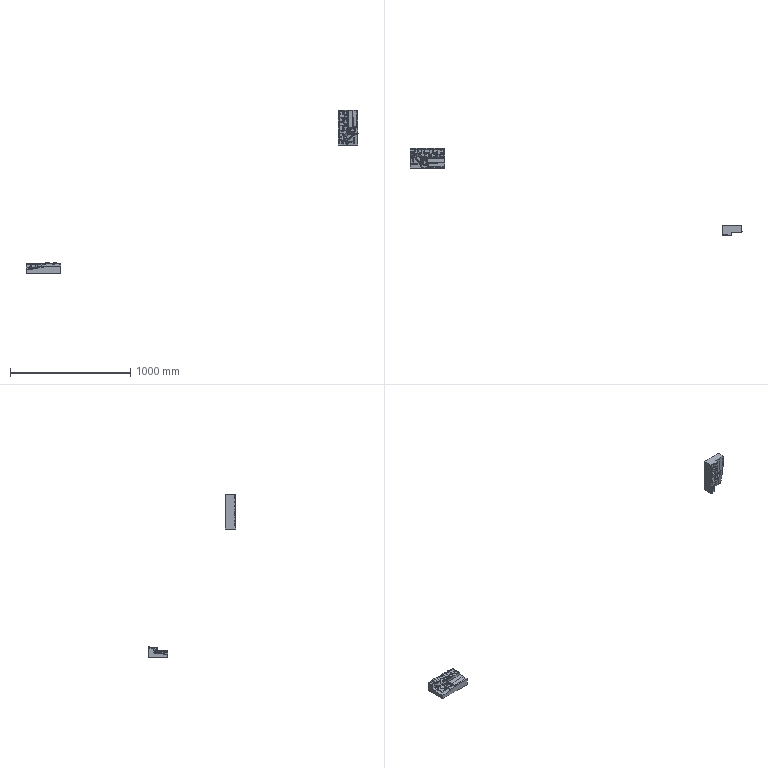NC program | NX | posted with a generic post | part box 2756 x 729.572 x 1353 mm
Lines 28320 to 29345 of 180527:
(CONTOUR_AREA , TOOL : B10)
N56626 M6
N56628 G54
N56630 G17 G0 G90 X35.48 Y166.497 B0. C0. S3000 M3
N56632 G43 Z10. H0
N56634 Z0.
N56636 G94 G1 Z-4.102 F2500.
N56638 X36.929 Z-4.118
N56640 X37.143 Z-3.988
N56642 X38.643 Z-3.197
N56644 X40.143 Z-2.553
N56646 X41.643 Z-2.051
N56648 X43.143 Z-1.669
N56650 X44.643 Z-1.416
N56652 X46.143 Z-1.275
N56654 X49.143 Z-1.261
N56656 X52.143 Z-1.295
N56658 X55.143 Z-1.329
N56660 X58.143 Z-1.363
N56662 X61.143 Z-1.397
N56664 X62.643 Z-1.472
N56666 X64.143 Z-1.658
N56668 X65.643 Z-1.962
N56670 X67.143 Z-2.389
N56672 X68.643 Z-2.946
N56674 X70.143 Z-3.648
N56676 X71.651 Z-4.513
N56678 X73.143 Z-4.527
N56680 X76.143 Z-4.554
N56682 X79.143 Z-4.582
N56684 X82.143 Z-4.609
N56686 X85.143 Z-4.636
N56688 X88.143 Z-4.658
N56690 X89.791 Z-4.669
N56692 X91.143 Z-3.943
N56694 X91.893 Z-3.62
N56696 X92.643 Z-3.368
N56698 X94.143 Z-3.051
N56700 X95.643 Z-2.951
N56702 X97.143 Z-2.899
N56704 X100.143 Z-2.794
N56706 X103.143 Z-2.689
N56708 X106.143 Z-2.584
N56710 X109.143 Z-2.479
N56712 X112.143 Z-2.374
N56714 X113.643 Z-2.321
N56716 X115.143 Z-2.344
N56718 X116.643 Z-2.59
N56720 X118.143 Z-3.015
N56722 X119.643 Z-3.57
N56724 X121.143 Z-4.268
N56726 X122.074 Z-4.782
N56728 X124.143 Z-4.78
N56730 X127.143 Z-4.777
N56732 X130.143 Z-4.775
N56734 X133.143 Z-4.772
N56736 X136.143 Z-4.764
N56738 X139.143 Z-4.755
N56740 X142.143 Z-4.746
N56742 X145.143 Z-4.733
N56744 X148.143 Z-4.717
N56746 X151.143 Z-4.702
N56748 X153.393 Z-4.691
N56750 X154.143 Z-4.668
N56752 X154.518 Z-4.517
N56754 X155.643 Z-3.508
N56756 X156.393 Z-2.935
N56758 X157.143 Z-2.443
N56760 X158.643 Z-1.654
N56762 X160.143 Z-1.097
N56764 X161.643 Z-0.737
N56766 X163.143 Z-0.56
N56768 X166.143 Z-0.475
N56770 X169.143 Z-0.401
N56772 X172.143 Z-0.333
N56774 X175.143 Z-0.266
N56776 X178.143 Z-0.204
N56778 X181.143 Z-0.144
N56780 X184.143 Z-0.085
N56782 X187.143 Z-0.027
N56784 X188.643 Z-0.001
N56786 X190.143 Z-0.078
N56788 X191.643 Z-0.328
N56790 X193.143 Z-0.762
N56792 X194.643 Z-1.408
N56794 X196.143 Z-2.302
N56796 X196.893 Z-2.858
N56798 X197.643 Z-3.51
N56800 X198.018 Z-3.87
N56802 X198.393 Z-4.171
N56804 X198.768 Z-4.281
N56806 X199.143 Z-4.283
N56808 X202.143 Z-4.269
N56810 X205.143 Z-4.26
N56812 X208.143 Z-4.251
N56814 X211.143 Z-4.242
N56816 X214.143 Z-4.232
N56818 X217.143 Z-4.223
N56820 X219.393 Z-4.215
N56822 X219.768 Z-4.122
N56824 X220.143 Z-3.84
N56826 X220.893 Z-3.116
N56828 X221.643 Z-2.476
N56830 X222.393 Z-1.935
N56832 X223.143 Z-1.484
N56834 X223.893 Z-1.112
N56836 X224.643 Z-0.809
N56838 X226.143 Z-0.378
N56840 X227.643 Z-0.165
N56842 X229.143 Z-0.144
N56844 X232.143 Z-0.177
N56846 X235.143 Z-0.211
N56848 X238.143 Z-0.25
N56850 X241.143 Z-0.289
N56852 X244.143 Z-0.332
N56854 X247.143 Z-0.379
N56856 X250.143 Z-0.426
N56858 X253.143 Z-0.474
N56860 X254.643 Z-0.515
N56862 X256.143 Z-0.727
N56864 X257.643 Z-1.164
N56866 X258.393 Z-1.469
N56868 X259.143 Z-1.842
N56870 X259.893 Z-2.294
N56872 X260.643 Z-2.836
N56874 X261.393 Z-3.481
N56876 X262.143 Z-4.212
N56878 X262.518 Z-4.441
N56880 X262.893 Z-4.497
N56882 X265.143 Z-4.53
N56884 X268.143 Z-4.577
N56886 X271.143 Z-4.624
N56888 X274.143 Z-4.672
N56890 X277.143 Z-4.719
N56892 X280.143 Z-4.767
N56894 X283.143
N56896 X286.143
N56898 X288.497 Z-4.768
N56900 X288.498 Y166.301
N56902 X286.143 Z-4.767
N56904 X283.143
N56906 X280.143
N56908 X277.143 Z-4.719
N56910 X274.143 Z-4.672
N56912 X271.143 Z-4.625
N56914 X268.143 Z-4.577
N56916 X265.143 Z-4.53
N56918 X263.643 Z-4.509
N56920 X262.893 Z-4.497
N56922 X262.518 Z-4.441
N56924 X262.143 Z-4.212
N56926 X261.393 Z-3.481
N56928 X260.643 Z-2.836
N56930 X259.893 Z-2.294
N56932 X259.143 Z-1.842
N56934 X258.393 Z-1.469
N56936 X257.643 Z-1.164
N56938 X256.143 Z-0.727
N56940 X254.643 Z-0.515
N56942 X253.143 Z-0.474
N56944 X250.143 Z-0.426
N56946 X247.143 Z-0.379
N56948 X244.143 Z-0.332
N56950 X241.143 Z-0.289
N56952 X238.143 Z-0.25
N56954 X235.143 Z-0.211
N56956 X232.143 Z-0.177
N56958 X229.143 Z-0.144
N56960 X227.643 Z-0.165
N56962 X226.143 Z-0.378
N56964 X224.643 Z-0.809
N56966 X223.893 Z-1.112
N56968 X223.143 Z-1.484
N56970 X222.393 Z-1.935
N56972 X221.643 Z-2.476
N56974 X220.893 Z-3.117
N56976 X220.143 Z-3.84
N56978 X219.768 Z-4.122
N56980 X219.393 Z-4.214
N56982 X218.643 Z-4.221
N56984 X217.143 Z-4.223
N56986 X214.143 Z-4.232
N56988 X211.143 Z-4.242
N56990 X208.143 Z-4.251
N56992 X205.143 Z-4.26
N56994 X202.143 Z-4.269
N56996 X199.143 Z-4.283
N56998 X198.768 Z-4.281
N57000 X198.393 Z-4.171
N57002 X198.018 Z-3.87
N57004 X197.643 Z-3.51
N57006 X196.893 Z-2.858
N57008 X196.143 Z-2.302
N57010 X194.643 Z-1.408
N57012 X193.143 Z-0.762
N57014 X191.643 Z-0.328
N57016 X190.143 Z-0.078
N57018 X188.643 Z-0.001
N57020 X187.143 Z-0.027
N57022 X184.143 Z-0.085
N57024 X181.143 Z-0.144
N57026 X178.143 Z-0.204
N57028 X175.143 Z-0.266
N57030 X172.143 Z-0.333
N57032 X169.143 Z-0.401
N57034 X166.143 Z-0.474
N57036 X163.143 Z-0.56
N57038 X161.643 Z-0.737
N57040 X160.143 Z-1.097
N57042 X158.643 Z-1.654
N57044 X157.143 Z-2.443
N57046 X156.393 Z-2.935
N57048 X155.643 Z-3.508
N57050 X154.893 Z-4.184
N57052 X154.518 Z-4.517
N57054 X154.143 Z-4.668
N57056 X153.393 Z-4.691
N57058 X152.643 Z-4.695
N57060 X151.143 Z-4.702
N57062 X148.143 Z-4.717
N57064 X145.143 Z-4.733
N57066 X142.143 Z-4.746
N57068 X139.143 Z-4.755
N57070 X136.143 Z-4.764
N57072 X133.143 Z-4.772
N57074 X130.143 Z-4.775
N57076 X127.143 Z-4.777
N57078 X124.143 Z-4.78
N57080 X122.074 Z-4.782
N57082 X121.143 Z-4.268
N57084 X119.643 Z-3.57
N57086 X118.143 Z-3.015
N57088 X116.643 Z-2.59
N57090 X115.143 Z-2.344
N57092 X113.643 Z-2.321
N57094 X112.143 Z-2.374
N57096 X109.143 Z-2.479
N57098 X106.143 Z-2.584
N57100 X103.143 Z-2.689
N57102 X100.143 Z-2.794
N57104 X97.143 Z-2.899
N57106 X95.643 Z-2.951
N57108 X94.143 Z-3.051
N57110 X92.643 Z-3.368
N57112 X91.893 Z-3.62
N57114 X91.143 Z-3.943
N57116 X89.791 Z-4.669
N57118 X88.143 Z-4.658
N57120 X85.143 Z-4.636
N57122 X82.143 Z-4.609
N57124 X79.143 Z-4.582
N57126 X76.143 Z-4.554
N57128 X73.143 Z-4.527
N57130 X71.651 Z-4.513
N57132 X70.143 Z-3.648
N57134 X68.643 Z-2.946
N57136 X67.143 Z-2.389
N57138 X65.643 Z-1.962
N57140 X64.143 Z-1.658
N57142 X62.643 Z-1.472
N57144 X61.143 Z-1.397
N57146 X58.143 Z-1.363
N57148 X55.143 Z-1.329
N57150 X52.143 Z-1.295
N57152 X49.143 Z-1.261
N57154 X46.143 Z-1.275
N57156 X44.643 Z-1.416
N57158 X43.143 Z-1.669
N57160 X41.643 Z-2.051
N57162 X40.143 Z-2.553
N57164 X38.643 Z-3.197
N57166 X37.143 Z-3.988
N57168 X36.929 Z-4.118
N57170 X34.143 Z-4.086
N57172 X31.143 Z-4.052
N57174 X28.143 Z-4.017
N57176 X25.143 Z-3.983
N57178 X22.143 Z-3.948
N57180 X19.143 Z-3.913
N57182 X16.143 Z-3.879
N57184 X13.143 Z-3.844
N57186 X10.143 Z-3.809
N57188 X7.143 Z-3.775
N57190 X4.143 Z-3.74
N57192 X1.143 Z-3.705
N57194 X-1.797 Z-3.671
N57196 X-1.857
N57198 Y166.103
N57200 X-1.797
N57202 X1.143 Z-3.705
N57204 X4.143 Z-3.74
N57206 X7.143 Z-3.775
N57208 X10.143 Z-3.809
N57210 X13.143 Z-3.844
N57212 X16.143 Z-3.879
N57214 X19.143 Z-3.913
N57216 X22.143 Z-3.948
N57218 X25.143 Z-3.983
N57220 X28.143 Z-4.017
N57222 X31.143 Z-4.052
N57224 X34.143 Z-4.086
N57226 X36.929 Z-4.118
N57228 X37.143 Z-3.988
N57230 X38.643 Z-3.197
N57232 X40.143 Z-2.553
N57234 X41.643 Z-2.051
N57236 X43.143 Z-1.669
N57238 X44.643 Z-1.416
N57240 X46.143 Z-1.275
N57242 X49.143 Z-1.261
N57244 X52.143 Z-1.295
N57246 X55.143 Z-1.329
N57248 X58.143 Z-1.363
N57250 X61.143 Z-1.397
N57252 X62.643 Z-1.472
N57254 X64.143 Z-1.658
N57256 X65.643 Z-1.962
N57258 X67.143 Z-2.389
N57260 X68.643 Z-2.946
N57262 X70.143 Z-3.648
N57264 X71.651 Z-4.513
N57266 X73.143 Z-4.527
N57268 X76.143 Z-4.554
N57270 X79.143 Z-4.582
N57272 X82.143 Z-4.609
N57274 X85.143 Z-4.636
N57276 X88.143 Z-4.658
N57278 X89.791 Z-4.669
N57280 X91.143 Z-3.943
N57282 X91.893 Z-3.62
N57284 X92.643 Z-3.368
N57286 X94.143 Z-3.051
N57288 X95.643 Z-2.951
N57290 X97.143 Z-2.899
N57292 X100.143 Z-2.794
N57294 X103.143 Z-2.689
N57296 X106.143 Z-2.584
N57298 X109.143 Z-2.479
N57300 X112.143 Z-2.374
N57302 X113.643 Z-2.321
N57304 X115.143 Z-2.344
N57306 X116.643 Z-2.59
N57308 X118.143 Z-3.015
N57310 X119.643 Z-3.57
N57312 X121.143 Z-4.268
N57314 X122.074 Z-4.782
N57316 X124.143 Z-4.78
N57318 X127.143 Z-4.777
N57320 X130.143 Z-4.775
N57322 X133.143 Z-4.772
N57324 X136.143 Z-4.764
N57326 X139.143 Z-4.755
N57328 X142.143 Z-4.746
N57330 X145.143 Z-4.733
N57332 X148.143 Z-4.717
N57334 X151.143 Z-4.702
N57336 X153.393 Z-4.691
N57338 X154.143 Z-4.668
N57340 X154.518 Z-4.517
N57342 X154.893 Z-4.184
N57344 X155.643 Z-3.508
N57346 X156.393 Z-2.935
N57348 X157.143 Z-2.443
N57350 X158.643 Z-1.654
N57352 X160.143 Z-1.097
N57354 X161.643 Z-0.737
N57356 X163.143 Z-0.56
N57358 X166.143 Z-0.474
N57360 X169.143 Z-0.401
N57362 X172.143 Z-0.333
N57364 X175.143 Z-0.266
N57366 X178.143 Z-0.204
N57368 X181.143 Z-0.144
N57370 X184.143 Z-0.085
N57372 X187.143 Z-0.027
N57374 X188.643 Z-0.001
N57376 X190.143 Z-0.078
N57378 X191.643 Z-0.328
N57380 X193.143 Z-0.762
N57382 X194.643 Z-1.408
N57384 X196.143 Z-2.302
N57386 X196.893 Z-2.858
N57388 X197.643 Z-3.51
N57390 X198.018 Z-3.87
N57392 X198.393 Z-4.171
N57394 X198.768 Z-4.281
N57396 X199.143 Z-4.283
N57398 X202.143 Z-4.269
N57400 X205.143 Z-4.26
N57402 X208.143 Z-4.251
N57404 X211.143 Z-4.242
N57406 X214.143 Z-4.232
N57408 X217.143 Z-4.223
N57410 X218.643 Z-4.221
N57412 X219.393 Z-4.214
N57414 X219.768 Z-4.122
N57416 X220.143 Z-3.84
N57418 X220.893 Z-3.117
N57420 X221.643 Z-2.476
N57422 X222.393 Z-1.935
N57424 X223.143 Z-1.484
N57426 X223.893 Z-1.112
N57428 X224.643 Z-0.809
N57430 X226.143 Z-0.378
N57432 X227.643 Z-0.165
N57434 X229.143 Z-0.144
N57436 X232.143 Z-0.177
N57438 X235.143 Z-0.211
N57440 X238.143 Z-0.25
N57442 X241.143 Z-0.288
N57444 X244.143 Z-0.332
N57446 X247.143 Z-0.379
N57448 X250.143 Z-0.426
N57450 X253.143 Z-0.474
N57452 X254.643 Z-0.515
N57454 X256.143 Z-0.727
N57456 X257.643 Z-1.164
N57458 X258.393 Z-1.469
N57460 X259.143 Z-1.842
N57462 X259.893 Z-2.294
N57464 X260.643 Z-2.836
N57466 X261.393 Z-3.481
N57468 X262.143 Z-4.212
N57470 X262.518 Z-4.441
N57472 X262.893 Z-4.497
N57474 X263.643 Z-4.509
N57476 X265.143 Z-4.53
N57478 X268.143 Z-4.577
N57480 X271.143 Z-4.625
N57482 X274.143 Z-4.672
N57484 X277.143 Z-4.719
N57486 X280.143 Z-4.766
N57488 X283.143 Z-4.767
N57490 X286.143
N57492 X288.498 Z-4.768
N57494 Y165.905
N57496 X286.143 Z-4.767
N57498 X283.143
N57500 X280.143 Z-4.766
N57502 X277.143 Z-4.719
N57504 X274.143 Z-4.672
N57506 X271.143 Z-4.625
N57508 X268.143 Z-4.577
N57510 X265.143 Z-4.53
N57512 X263.643 Z-4.509
N57514 X262.893 Z-4.497
N57516 X262.518 Z-4.441
N57518 X262.143 Z-4.212
N57520 X261.393 Z-3.481
N57522 X260.643 Z-2.836
N57524 X259.893 Z-2.294
N57526 X259.143 Z-1.842
N57528 X258.393 Z-1.469
N57530 X257.643 Z-1.164
N57532 X256.143 Z-0.727
N57534 X254.643 Z-0.515
N57536 X253.143 Z-0.474
N57538 X250.143 Z-0.426
N57540 X247.143 Z-0.379
N57542 X244.143 Z-0.332
N57544 X241.143 Z-0.288
N57546 X238.143 Z-0.25
N57548 X235.143 Z-0.211
N57550 X232.143 Z-0.177
N57552 X229.143 Z-0.144
N57554 X227.643 Z-0.165
N57556 X226.143 Z-0.378
N57558 X224.643 Z-0.809
N57560 X223.893 Z-1.112
N57562 X223.143 Z-1.484
N57564 X222.393 Z-1.935
N57566 X221.643 Z-2.476
N57568 X220.893 Z-3.117
N57570 X220.143 Z-3.84
N57572 X219.768 Z-4.122
N57574 X219.393 Z-4.214
N57576 X218.643 Z-4.221
N57578 X217.143 Z-4.223
N57580 X214.143 Z-4.232
N57582 X211.143 Z-4.242
N57584 X208.143 Z-4.251
N57586 X205.143 Z-4.26
N57588 X202.143 Z-4.269
N57590 X199.143 Z-4.283
N57592 X198.768 Z-4.281
N57594 X198.393 Z-4.171
N57596 X198.018 Z-3.87
N57598 X197.643 Z-3.51
N57600 X196.893 Z-2.858
N57602 X196.143 Z-2.302
N57604 X194.643 Z-1.408
N57606 X193.143 Z-0.762
N57608 X191.643 Z-0.328
N57610 X190.143 Z-0.078
N57612 X188.643 Z-0.001
N57614 X187.143 Z-0.027
N57616 X184.143 Z-0.085
N57618 X181.143 Z-0.144
N57620 X178.143 Z-0.204
N57622 X175.143 Z-0.266
N57624 X172.143 Z-0.333
N57626 X169.143 Z-0.401
N57628 X166.143 Z-0.474
N57630 X163.143 Z-0.56
N57632 X161.643 Z-0.737
N57634 X160.143 Z-1.097
N57636 X158.643 Z-1.654
N57638 X157.143 Z-2.443
N57640 X156.393 Z-2.935
N57642 X155.643 Z-3.508
N57644 X154.893 Z-4.184
N57646 X154.518 Z-4.517
N57648 X154.143 Z-4.668
N57650 X153.393 Z-4.691
N57652 X151.143 Z-4.702
N57654 X148.143 Z-4.717
N57656 X145.143 Z-4.733
N57658 X142.143 Z-4.746
N57660 X139.143 Z-4.755
N57662 X136.143 Z-4.764
N57664 X133.143 Z-4.772
N57666 X130.143 Z-4.775
N57668 X127.143 Z-4.777
N57670 X124.143 Z-4.78
N57672 X122.074 Z-4.782
N57674 X121.143 Z-4.268
N57676 X119.643 Z-3.57
N57678 X118.143 Z-3.015
N57680 X116.643 Z-2.59
N57682 X115.143 Z-2.344
N57684 X113.643 Z-2.321
N57686 X112.143 Z-2.374
N57688 X109.143 Z-2.479
N57690 X106.143 Z-2.584
N57692 X103.143 Z-2.689
N57694 X100.143 Z-2.794
N57696 X97.143 Z-2.899
N57698 X95.643 Z-2.951
N57700 X94.143 Z-3.051
N57702 X92.643 Z-3.368
N57704 X91.893 Z-3.62
N57706 X91.143 Z-3.943
N57708 X89.791 Z-4.669
N57710 X88.143 Z-4.658
N57712 X85.143 Z-4.636
N57714 X82.143 Z-4.609
N57716 X79.143 Z-4.582
N57718 X76.143 Z-4.554
N57720 X73.143 Z-4.527
N57722 X71.651 Z-4.513
N57724 X70.143 Z-3.648
N57726 X68.643 Z-2.946
N57728 X67.143 Z-2.389
N57730 X65.643 Z-1.962
N57732 X64.143 Z-1.658
N57734 X62.643 Z-1.472
N57736 X61.143 Z-1.397
N57738 X58.143 Z-1.363
N57740 X55.143 Z-1.329
N57742 X52.143 Z-1.295
N57744 X49.143 Z-1.26
N57746 X46.143 Z-1.275
N57748 X44.643 Z-1.416
N57750 X43.143 Z-1.669
N57752 X41.643 Z-2.051
N57754 X40.143 Z-2.553
N57756 X38.643 Z-3.197
N57758 X37.143 Z-3.988
N57760 X36.929 Z-4.118
N57762 X34.143 Z-4.086
N57764 X31.143 Z-4.052
N57766 X28.143 Z-4.017
N57768 X25.143 Z-3.983
N57770 X22.143 Z-3.948
N57772 X19.143 Z-3.913
N57774 X16.143 Z-3.879
N57776 X13.143 Z-3.844
N57778 X10.143 Z-3.809
N57780 X7.143 Z-3.775
N57782 X4.143 Z-3.74
N57784 X1.143 Z-3.705
N57786 X-1.797 Z-3.671
N57788 X-1.857
N57790 Y165.706
N57792 X-1.797
N57794 X1.143 Z-3.705
N57796 X4.143 Z-3.74
N57798 X7.143 Z-3.775
N57800 X10.143 Z-3.809
N57802 X13.143 Z-3.844
N57804 X16.143 Z-3.879
N57806 X19.143 Z-3.913
N57808 X22.143 Z-3.948
N57810 X25.143 Z-3.983
N57812 X28.143 Z-4.017
N57814 X31.143 Z-4.052
N57816 X34.143 Z-4.086
N57818 X35.536 Z-4.102
N57820 X36.929 Z-4.118
N57822 X37.143 Z-3.988
N57824 X38.643 Z-3.197
N57826 X40.143 Z-2.553
N57828 X41.643 Z-2.051
N57830 X43.143 Z-1.669
N57832 X44.643 Z-1.416
N57834 X46.143 Z-1.275
N57836 X49.143 Z-1.26
N57838 X52.143 Z-1.295
N57840 X55.143 Z-1.329
N57842 X58.143 Z-1.363
N57844 X61.143 Z-1.397
N57846 X62.643 Z-1.472
N57848 X64.143 Z-1.658
N57850 X65.643 Z-1.962
N57852 X67.143 Z-2.389
N57854 X68.643 Z-2.946
N57856 X70.143 Z-3.648
N57858 X71.651 Z-4.513
N57860 X73.143 Z-4.527
N57862 X76.143 Z-4.554
N57864 X79.143 Z-4.582
N57866 X82.143 Z-4.609
N57868 X85.143 Z-4.636
N57870 X88.143 Z-4.658
N57872 X88.967 Z-4.664
N57874 X89.791 Z-4.669
N57876 X91.143 Z-3.943
N57878 X91.893 Z-3.62
N57880 X92.643 Z-3.368
N57882 X94.143 Z-3.051
N57884 X95.643 Z-2.951
N57886 X97.143 Z-2.899
N57888 X100.143 Z-2.794
N57890 X103.143 Z-2.689
N57892 X106.143 Z-2.584
N57894 X109.143 Z-2.479
N57896 X112.143 Z-2.374
N57898 X113.643 Z-2.321
N57900 X115.143 Z-2.344
N57902 X116.643 Z-2.59
N57904 X118.143 Z-3.015
N57906 X119.643 Z-3.57
N57908 X121.143 Z-4.268
N57910 X122.074 Z-4.782
N57912 X123.108 Z-4.781
N57914 X124.143 Z-4.78
N57916 X127.143 Z-4.777
N57918 X130.143 Z-4.775
N57920 X133.143 Z-4.772
N57922 X136.143 Z-4.764
N57924 X139.143 Z-4.755
N57926 X142.143 Z-4.746
N57928 X145.143 Z-4.733
N57930 X148.143 Z-4.717
N57932 X151.143 Z-4.702
N57934 X153.393 Z-4.691
N57936 X154.143 Z-4.668
N57938 X154.518 Z-4.517
N57940 X154.893 Z-4.184
N57942 X155.643 Z-3.508
N57944 X156.393 Z-2.935
N57946 X157.143 Z-2.443
N57948 X158.643 Z-1.654
N57950 X160.143 Z-1.097
N57952 X161.643 Z-0.737
N57954 X163.143 Z-0.56
N57956 X166.143 Z-0.474
N57958 X169.143 Z-0.401
N57960 X172.143 Z-0.333
N57962 X175.143 Z-0.266
N57964 X178.143 Z-0.204
N57966 X181.143 Z-0.144
N57968 X184.143 Z-0.085
N57970 X187.143 Z-0.027
N57972 X188.643 Z-0.001
N57974 X190.143 Z-0.078
N57976 X191.643 Z-0.328
N57978 X193.143 Z-0.762
N57980 X194.643 Z-1.408
N57982 X196.143 Z-2.302
N57984 X196.893 Z-2.857
N57986 X197.643 Z-3.51
N57988 X198.018 Z-3.87
N57990 X198.393 Z-4.171
N57992 X198.768 Z-4.281
N57994 X199.143 Z-4.283
N57996 X202.143 Z-4.269
N57998 X205.143 Z-4.26
N58000 X208.143 Z-4.251
N58002 X211.143 Z-4.242
N58004 X214.143 Z-4.232
N58006 X217.143 Z-4.223
N58008 X218.643 Z-4.221
N58010 X219.393 Z-4.214
N58012 X219.768 Z-4.122
N58014 X220.143 Z-3.84
N58016 X220.893 Z-3.117
N58018 X221.643 Z-2.476
N58020 X222.393 Z-1.935
N58022 X223.143 Z-1.484
N58024 X223.893 Z-1.112
N58026 X224.643 Z-0.809
N58028 X226.143 Z-0.378
N58030 X227.643 Z-0.165
N58032 X229.143 Z-0.144
N58034 X232.143 Z-0.177
N58036 X235.143 Z-0.211
N58038 X238.143 Z-0.25
N58040 X241.143 Z-0.288
N58042 X244.143 Z-0.332
N58044 X247.143 Z-0.379
N58046 X250.143 Z-0.426
N58048 X253.143 Z-0.474
N58050 X254.643 Z-0.515
N58052 X256.143 Z-0.727
N58054 X257.643 Z-1.164
N58056 X258.393 Z-1.469
N58058 X259.143 Z-1.842
N58060 X259.893 Z-2.294
N58062 X260.643 Z-2.836
N58064 X261.393 Z-3.481
N58066 X262.143 Z-4.212
N58068 X262.518 Z-4.441
N58070 X262.893 Z-4.497
N58072 X263.643 Z-4.509
N58074 X265.143 Z-4.53
N58076 X268.143 Z-4.577
N58078 X271.143 Z-4.625
N58080 X274.143 Z-4.672
N58082 X277.143 Z-4.719
N58084 X280.143 Z-4.766
N58086 X283.143 Z-4.767
N58088 X286.143
N58090 X288.498 Z-4.768
N58092 Y165.508
N58094 X286.143 Z-4.767
N58096 X283.143
N58098 X280.143 Z-4.766
N58100 X277.143 Z-4.719
N58102 X274.143 Z-4.672
N58104 X271.143 Z-4.625
N58106 X268.143 Z-4.577
N58108 X265.143 Z-4.53
N58110 X263.643 Z-4.509
N58112 X262.893 Z-4.497
N58114 X262.518 Z-4.441
N58116 X262.143 Z-4.212
N58118 X261.393 Z-3.481
N58120 X260.643 Z-2.836
N58122 X259.893 Z-2.294
N58124 X259.143 Z-1.842
N58126 X258.393 Z-1.469
N58128 X257.643 Z-1.164
N58130 X256.143 Z-0.727
N58132 X254.643 Z-0.516
N58134 X253.143 Z-0.474
N58136 X250.143 Z-0.426
N58138 X247.143 Z-0.379
N58140 X244.143 Z-0.332
N58142 X241.143 Z-0.288
N58144 X238.143 Z-0.25
N58146 X235.143 Z-0.211
N58148 X232.143 Z-0.177
N58150 X229.143 Z-0.144
N58152 X227.643 Z-0.165
N58154 X226.143 Z-0.378
N58156 X224.643 Z-0.809
N58158 X223.893 Z-1.112
N58160 X223.143 Z-1.484
N58162 X222.393 Z-1.935
N58164 X221.643 Z-2.476
N58166 X220.893 Z-3.117
N58168 X220.143 Z-3.84
N58170 X219.768 Z-4.122
N58172 X219.393 Z-4.214
N58174 X218.643 Z-4.221
N58176 X217.143 Z-4.223
N58178 X214.143 Z-4.232
N58180 X211.143 Z-4.242
N58182 X208.143 Z-4.251
N58184 X205.143 Z-4.26
N58186 X202.143 Z-4.269
N58188 X199.143 Z-4.283
N58190 X198.768 Z-4.281
N58192 X198.393 Z-4.171
N58194 X198.018 Z-3.87
N58196 X197.643 Z-3.51
N58198 X196.893 Z-2.857
N58200 X196.143 Z-2.302
N58202 X194.643 Z-1.408
N58204 X193.143 Z-0.762
N58206 X191.643 Z-0.328
N58208 X190.143 Z-0.078
N58210 X188.643 Z-0.001
N58212 X187.143 Z-0.027
N58214 X184.143 Z-0.085
N58216 X181.143 Z-0.144
N58218 X178.143 Z-0.204
N58220 X175.143 Z-0.266
N58222 X172.143 Z-0.333
N58224 X169.143 Z-0.401
N58226 X166.143 Z-0.474
N58228 X163.143 Z-0.56
N58230 X161.643 Z-0.737
N58232 X160.143 Z-1.097
N58234 X158.643 Z-1.654
N58236 X157.143 Z-2.443
N58238 X156.393 Z-2.935
N58240 X155.643 Z-3.508
N58242 X154.893 Z-4.184
N58244 X154.518 Z-4.517
N58246 X154.143 Z-4.668
N58248 X153.393 Z-4.691
N58250 X151.143 Z-4.702
N58252 X148.143 Z-4.717
N58254 X145.143 Z-4.733
N58256 X142.143 Z-4.746
N58258 X139.143 Z-4.755
N58260 X136.143 Z-4.764
N58262 X133.143 Z-4.772
N58264 X130.143 Z-4.775
N58266 X127.143 Z-4.777
N58268 X124.143 Z-4.78
N58270 X122.074 Z-4.782
N58272 X121.143 Z-4.268
N58274 X119.643 Z-3.57
N58276 X118.143 Z-3.015
N58278 X116.643 Z-2.59
N58280 X115.143 Z-2.344
N58282 X113.643 Z-2.321
N58284 X112.143 Z-2.374
N58286 X109.143 Z-2.479
N58288 X106.143 Z-2.584
N58290 X103.143 Z-2.689
N58292 X100.143 Z-2.794
N58294 X97.143 Z-2.899
N58296 X95.643 Z-2.951
N58298 X94.143 Z-3.051
N58300 X92.643 Z-3.368
N58302 X91.893 Z-3.62
N58304 X91.143 Z-3.943
N58306 X89.791 Z-4.669
N58308 X88.143 Z-4.658
N58310 X85.143 Z-4.636
N58312 X82.143 Z-4.609
N58314 X79.143 Z-4.582
N58316 X76.143 Z-4.554
N58318 X73.143 Z-4.527
N58320 X71.651 Z-4.513
N58322 X70.143 Z-3.648
N58324 X68.643 Z-2.946
N58326 X67.143 Z-2.389
N58328 X65.643 Z-1.962
N58330 X64.143 Z-1.658
N58332 X62.643 Z-1.472
N58334 X61.143 Z-1.397
N58336 X58.143 Z-1.363
N58338 X55.143 Z-1.329
N58340 X52.143 Z-1.295
N58342 X49.143 Z-1.26
N58344 X46.143 Z-1.275
N58346 X44.643 Z-1.416
N58348 X43.143 Z-1.669
N58350 X41.643 Z-2.051
N58352 X40.143 Z-2.553
N58354 X38.643 Z-3.197
N58356 X37.143 Z-3.988
N58358 X36.928 Z-4.118
N58360 X34.143 Z-4.086
N58362 X31.143 Z-4.052
N58364 X28.143 Z-4.017
N58366 X25.143 Z-3.983
N58368 X22.143 Z-3.948
N58370 X19.143 Z-3.913
N58372 X16.143 Z-3.879
N58374 X13.143 Z-3.844
N58376 X10.143 Z-3.809
N58378 X7.143 Z-3.775
N58380 X4.143 Z-3.74
N58382 X1.143 Z-3.705
N58384 X-1.797 Z-3.671
N58386 X-1.857
N58388 Y165.309
N58390 X-1.797
N58392 X1.143 Z-3.705
N58394 X4.143 Z-3.74
N58396 X7.143 Z-3.775
N58398 X10.143 Z-3.809
N58400 X13.143 Z-3.844
N58402 X16.143 Z-3.879
N58404 X19.143 Z-3.913
N58406 X22.143 Z-3.948
N58408 X25.143 Z-3.983
N58410 X28.143 Z-4.017
N58412 X31.143 Z-4.052
N58414 X34.143 Z-4.086
N58416 X36.928 Z-4.118
N58418 X37.143 Z-3.988
N58420 X38.643 Z-3.197
N58422 X40.143 Z-2.553
N58424 X41.643 Z-2.051
N58426 X43.143 Z-1.669
N58428 X44.643 Z-1.415
N58430 X46.143 Z-1.274
N58432 X49.143 Z-1.26
N58434 X52.143 Z-1.294
N58436 X55.143 Z-1.329
N58438 X58.143 Z-1.363
N58440 X61.143 Z-1.397
N58442 X62.643 Z-1.472
N58444 X64.143 Z-1.658
N58446 X65.643 Z-1.962
N58448 X67.143 Z-2.389
N58450 X68.643 Z-2.946
N58452 X70.143 Z-3.648
N58454 X71.652 Z-4.514
N58456 X73.143 Z-4.527
N58458 X76.143 Z-4.554
N58460 X79.143 Z-4.582
N58462 X82.143 Z-4.609
N58464 X85.143 Z-4.636
N58466 X88.143 Z-4.658
N58468 X89.791 Z-4.67
N58470 X91.143 Z-3.943
N58472 X91.893 Z-3.62
N58474 X92.643 Z-3.367
N58476 X94.143 Z-3.051
N58478 X95.643 Z-2.951
N58480 X97.143 Z-2.899
N58482 X100.143 Z-2.794
N58484 X103.143 Z-2.689
N58486 X106.143 Z-2.584
N58488 X109.143 Z-2.479
N58490 X112.143 Z-2.374
N58492 X113.643 Z-2.321
N58494 X115.143 Z-2.344
N58496 X116.643 Z-2.589
N58498 X118.143 Z-3.015
N58500 X119.643 Z-3.57
N58502 X121.143 Z-4.268
N58504 X122.075 Z-4.782
N58506 X124.143 Z-4.78
N58508 X127.143 Z-4.777
N58510 X130.143 Z-4.775
N58512 X133.143 Z-4.772
N58514 X136.143 Z-4.764
N58516 X139.143 Z-4.755
N58518 X142.143 Z-4.746
N58520 X145.143 Z-4.733
N58522 X148.143 Z-4.718
N58524 X151.143 Z-4.702
N58526 X152.643 Z-4.695
N58528 X153.393 Z-4.691
N58530 X154.143 Z-4.668
N58532 X154.518 Z-4.518
N58534 X154.893 Z-4.184
N58536 X155.643 Z-3.508
N58538 X156.393 Z-2.935
N58540 X157.143 Z-2.443
N58542 X158.643 Z-1.654
N58544 X160.143 Z-1.097
N58546 X161.643 Z-0.737
N58548 X163.143 Z-0.559
N58550 X166.143 Z-0.474
N58552 X169.143 Z-0.401
N58554 X172.143 Z-0.333
N58556 X175.143 Z-0.266
N58558 X178.143 Z-0.204
N58560 X181.143 Z-0.144
N58562 X184.143 Z-0.085
N58564 X187.143 Z-0.027
N58566 X188.643 Z-0.001
N58568 X190.143 Z-0.077
N58570 X191.643 Z-0.328
N58572 X193.143 Z-0.762
N58574 X194.643 Z-1.408
N58576 X196.143 Z-2.302
N58578 X196.893 Z-2.857
N58580 X197.643 Z-3.51
N58582 X198.018 Z-3.87
N58584 X198.393 Z-4.172
N58586 X198.768 Z-4.281
N58588 X199.143 Z-4.283
N58590 X202.143 Z-4.269
N58592 X205.143 Z-4.26
N58594 X208.143 Z-4.251
N58596 X211.143 Z-4.241
N58598 X214.143 Z-4.232
N58600 X217.143 Z-4.223
N58602 X218.643 Z-4.221
N58604 X219.393 Z-4.215
N58606 X219.768 Z-4.122
N58608 X220.143 Z-3.84
N58610 X220.893 Z-3.117
N58612 X221.643 Z-2.475
N58614 X222.393 Z-1.935
N58616 X223.143 Z-1.484
N58618 X223.893 Z-1.111
N58620 X224.643 Z-0.809
N58622 X226.143 Z-0.377
N58624 X227.643 Z-0.165
N58626 X229.143 Z-0.144
N58628 X232.143 Z-0.177
N58630 X235.143 Z-0.211
N58632 X238.143 Z-0.25
N58634 X241.143 Z-0.288
N58636 X244.143 Z-0.332
N58638 X247.143 Z-0.379
N58640 X250.143 Z-0.426
N58642 X253.143 Z-0.474
N58644 X254.643 Z-0.515
N58646 X256.143 Z-0.727
N58648 X257.643 Z-1.163
N58650 X258.393 Z-1.469
N58652 X259.143 Z-1.842
N58654 X259.893 Z-2.293
N58656 X260.643 Z-2.836
N58658 X261.393 Z-3.48
N58660 X262.143 Z-4.212
N58662 X262.518 Z-4.442
N58664 X262.893 Z-4.497
N58666 X263.643 Z-4.509
N58668 X265.143 Z-4.53
N58670 X268.143 Z-4.577